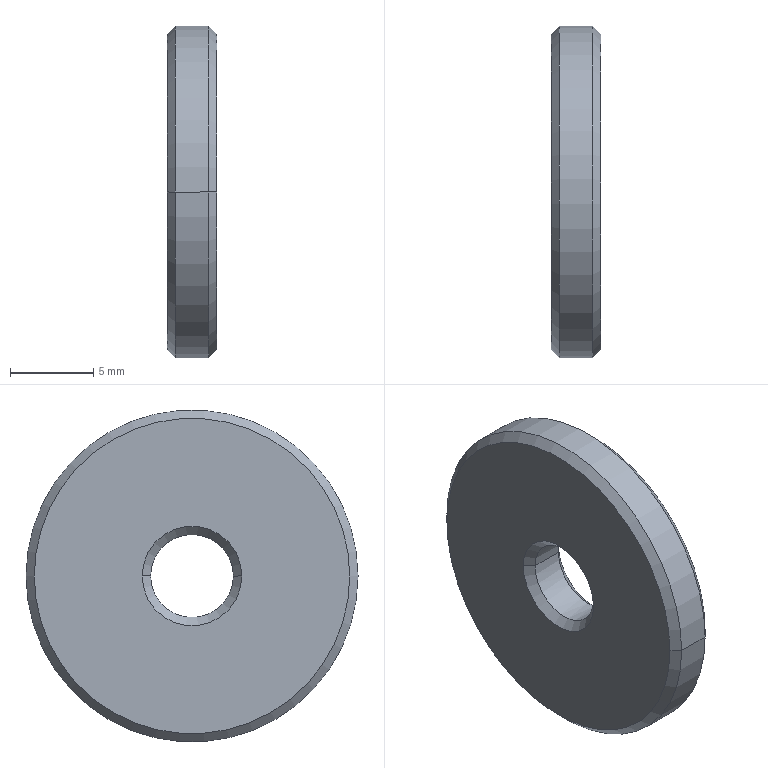Part | STEP file | wssb20_5_3_2_03 | 1 solid | 14 faces | box 3 x 20 x 20 mm | volume 863.938 mm3 | cone 8 | cylinder 4 | plane 2 | commonest cylinder face diameters 5 x2 20 x2
STEP:
#1=CARTESIAN_POINT('',(0.,0.,0.));
#2=DIRECTION('',(0.,0.,1.));
#3=DIRECTION('',(1.,0.,0.));
#4=AXIS2_PLACEMENT_3D('',#1,#2,#3);
#5=CARTESIAN_POINT('',(0.5,-2.5,0.));
#6=VERTEX_POINT('',#5);
#7=CARTESIAN_POINT('',(0.,-3.,0.));
#8=VERTEX_POINT('',#7);
#9=CARTESIAN_POINT('',(0.,-3.,0.));
#10=DIRECTION('',(-0.7071,-0.7071,0.));
#11=VECTOR('',#10,1.);
#12=LINE('',#9,#11);
#13=CARTESIAN_POINT('',(0.,0.,0.));
#14=DIRECTION('',(-1.,0.,0.));
#15=DIRECTION('',(0.,-1.,0.));
#16=AXIS2_PLACEMENT_3D('',#13,#14,#15);
#17=CONICAL_SURFACE('',#16,3.,0.7854);
#18=CARTESIAN_POINT('',(6.283,0.));
#19=DIRECTION('',(0.,1.));
#20=VECTOR('',#19,1.);
#21=LINE('',#18,#20);
#22=(GEOMETRIC_REPRESENTATION_CONTEXT(2)PARAMETRIC_REPRESENTATION_CONTEXT()REPRESENTATION_CONTEXT('',''));
#23=DEFINITIONAL_REPRESENTATION('',(#21),#22);
#24=PCURVE('',#17,#23);
#25=CARTESIAN_POINT('',(0.,0.,0.));
#26=DIRECTION('',(-1.,0.,0.));
#27=DIRECTION('',(0.,-1.,0.));
#28=AXIS2_PLACEMENT_3D('',#25,#26,#27);
#29=CONICAL_SURFACE('',#28,3.,0.7854);
#30=CARTESIAN_POINT('',(0.,0.));
#31=DIRECTION('',(0.,1.));
#32=VECTOR('',#31,1.);
#33=LINE('',#30,#32);
#34=(GEOMETRIC_REPRESENTATION_CONTEXT(2)PARAMETRIC_REPRESENTATION_CONTEXT()REPRESENTATION_CONTEXT('',''));
#35=DEFINITIONAL_REPRESENTATION('',(#33),#34);
#36=PCURVE('',#29,#35);
#37=SURFACE_CURVE('',#12,(#24,#36),.PCURVE_S1.);
#38=EDGE_CURVE('',#6,#8,#37,.T.);
#39=ORIENTED_EDGE('',*,*,#38,.T.);
#40=CARTESIAN_POINT('',(0.,3.,0.));
#41=VERTEX_POINT('',#40);
#42=CARTESIAN_POINT('',(0.,0.,0.));
#43=DIRECTION('',(1.,0.,0.));
#44=DIRECTION('',(0.,-1.,0.));
#45=AXIS2_PLACEMENT_3D('',#42,#43,#44);
#46=CIRCLE('',#45,3.);
#47=CARTESIAN_POINT('',(6.283,0.));
#48=DIRECTION('',(-1.,0.));
#49=VECTOR('',#48,1.);
#50=LINE('',#47,#49);
#51=(GEOMETRIC_REPRESENTATION_CONTEXT(2)PARAMETRIC_REPRESENTATION_CONTEXT()REPRESENTATION_CONTEXT('',''));
#52=DEFINITIONAL_REPRESENTATION('',(#50),#51);
#53=PCURVE('',#17,#52);
#54=CARTESIAN_POINT('',(0.,-6.25,0.));
#55=DIRECTION('',(-1.,0.,0.));
#56=DIRECTION('',(0.,-1.,0.));
#57=AXIS2_PLACEMENT_3D('',#54,#55,#56);
#58=PLANE('',#57);
#59=CARTESIAN_POINT('',(-3.25,0.));
#60=CARTESIAN_POINT('',(-3.25,-5.196));
#61=CARTESIAN_POINT('',(-7.75,-2.598));
#62=CARTESIAN_POINT('',(-12.25,0.));
#63=CARTESIAN_POINT('',(-7.75,2.598));
#64=CARTESIAN_POINT('',(-3.25,5.196));
#65=CARTESIAN_POINT('',(-3.25,0.));
#66=(BOUNDED_CURVE()B_SPLINE_CURVE(2,(#59,#60,#61,#62,#63,#64,#65),.UNSPECIFIED.,.T.,.F.)B_SPLINE_CURVE_WITH_KNOTS((1,2,2,2,2,1),(-2.094,0.,2.094,4.189,6.283,8.378),.UNSPECIFIED.)CURVE()GEOMETRIC_REPRESENTATION_ITEM()RATIONAL_B_SPLINE_CURVE((1.,0.5,1.,0.5,1.,0.5,1.))REPRESENTATION_ITEM(''));
#67=(GEOMETRIC_REPRESENTATION_CONTEXT(2)PARAMETRIC_REPRESENTATION_CONTEXT()REPRESENTATION_CONTEXT('',''));
#68=DEFINITIONAL_REPRESENTATION('',(#66),#67);
#69=PCURVE('',#58,#68);
#70=SURFACE_CURVE('',#46,(#53,#69),.PCURVE_S1.);
#71=EDGE_CURVE('',#8,#41,#70,.T.);
#72=ORIENTED_EDGE('',*,*,#71,.T.);
#73=CARTESIAN_POINT('',(0.5,2.5,0.));
#74=VERTEX_POINT('',#73);
#75=CARTESIAN_POINT('',(0.,3.,0.));
#76=DIRECTION('',(-0.7071,0.7071,0.));
#77=VECTOR('',#76,1.);
#78=LINE('',#75,#77);
#79=CARTESIAN_POINT('',(3.142,0.));
#80=DIRECTION('',(0.,1.));
#81=VECTOR('',#80,1.);
#82=LINE('',#79,#81);
#83=(GEOMETRIC_REPRESENTATION_CONTEXT(2)PARAMETRIC_REPRESENTATION_CONTEXT()REPRESENTATION_CONTEXT('',''));
#84=DEFINITIONAL_REPRESENTATION('',(#82),#83);
#85=PCURVE('',#17,#84);
#86=CARTESIAN_POINT('',(3.142,0.));
#87=DIRECTION('',(0.,1.));
#88=VECTOR('',#87,1.);
#89=LINE('',#86,#88);
#90=(GEOMETRIC_REPRESENTATION_CONTEXT(2)PARAMETRIC_REPRESENTATION_CONTEXT()REPRESENTATION_CONTEXT('',''));
#91=DEFINITIONAL_REPRESENTATION('',(#89),#90);
#92=PCURVE('',#29,#91);
#93=SURFACE_CURVE('',#78,(#85,#92),.PCURVE_S1.);
#94=EDGE_CURVE('',#74,#41,#93,.T.);
#95=ORIENTED_EDGE('',*,*,#94,.F.);
#96=CARTESIAN_POINT('',(0.5,0.,0.));
#97=DIRECTION('',(-1.,0.,0.));
#98=DIRECTION('',(0.,-1.,0.));
#99=AXIS2_PLACEMENT_3D('',#96,#97,#98);
#100=CIRCLE('',#99,2.5);
#101=CARTESIAN_POINT('',(0.,-0.5));
#102=DIRECTION('',(1.,0.));
#103=VECTOR('',#102,1.);
#104=LINE('',#101,#103);
#105=(GEOMETRIC_REPRESENTATION_CONTEXT(2)PARAMETRIC_REPRESENTATION_CONTEXT()REPRESENTATION_CONTEXT('',''));
#106=DEFINITIONAL_REPRESENTATION('',(#104),#105);
#107=PCURVE('',#17,#106);
#108=CARTESIAN_POINT('',(1.5,0.,0.));
#109=DIRECTION('',(-1.,0.,0.));
#110=DIRECTION('',(0.,-1.,0.));
#111=AXIS2_PLACEMENT_3D('',#108,#109,#110);
#112=CYLINDRICAL_SURFACE('',#111,2.5);
#113=CARTESIAN_POINT('',(0.,1.));
#114=DIRECTION('',(1.,0.));
#115=VECTOR('',#114,1.);
#116=LINE('',#113,#115);
#117=(GEOMETRIC_REPRESENTATION_CONTEXT(2)PARAMETRIC_REPRESENTATION_CONTEXT()REPRESENTATION_CONTEXT('',''));
#118=DEFINITIONAL_REPRESENTATION('',(#116),#117);
#119=PCURVE('',#112,#118);
#120=SURFACE_CURVE('',#100,(#107,#119),.PCURVE_S1.);
#121=EDGE_CURVE('',#74,#6,#120,.T.);
#122=ORIENTED_EDGE('',*,*,#121,.T.);
#123=EDGE_LOOP('',(#39,#72,#95,#122));
#124=FACE_BOUND('',#123,.F.);
#125=ADVANCED_FACE('',(#124),#17,.F.);
#126=CARTESIAN_POINT('',(0.,-9.5,0.));
#127=VERTEX_POINT('',#126);
#128=CARTESIAN_POINT('',(0.,9.5,0.));
#129=VERTEX_POINT('',#128);
#130=CARTESIAN_POINT('',(0.,0.,0.));
#131=DIRECTION('',(-1.,0.,0.));
#132=DIRECTION('',(0.,1.,0.));
#133=AXIS2_PLACEMENT_3D('',#130,#131,#132);
#134=CIRCLE('',#133,9.5);
#135=CARTESIAN_POINT('',(0.5,0.,0.));
#136=DIRECTION('',(1.,0.,0.));
#137=DIRECTION('',(0.,1.,0.));
#138=AXIS2_PLACEMENT_3D('',#135,#136,#137);
#139=CONICAL_SURFACE('',#138,10.,0.7854);
#140=CARTESIAN_POINT('',(6.283,-0.5));
#141=DIRECTION('',(-1.,0.));
#142=VECTOR('',#141,1.);
#143=LINE('',#140,#142);
#144=(GEOMETRIC_REPRESENTATION_CONTEXT(2)PARAMETRIC_REPRESENTATION_CONTEXT()REPRESENTATION_CONTEXT('',''));
#145=DEFINITIONAL_REPRESENTATION('',(#143),#144);
#146=PCURVE('',#139,#145);
#147=CARTESIAN_POINT('',(-6.25,0.));
#148=DIRECTION('',(-1.,0.));
#149=AXIS2_PLACEMENT_2D('',#147,#148);
#150=CIRCLE('',#149,9.5);
#151=(GEOMETRIC_REPRESENTATION_CONTEXT(2)PARAMETRIC_REPRESENTATION_CONTEXT()REPRESENTATION_CONTEXT('',''));
#152=DEFINITIONAL_REPRESENTATION('',(#150),#151);
#153=PCURVE('',#58,#152);
#154=SURFACE_CURVE('',#134,(#146,#153),.PCURVE_S1.);
#155=EDGE_CURVE('',#127,#129,#154,.T.);
#156=ORIENTED_EDGE('',*,*,#155,.F.);
#157=CARTESIAN_POINT('',(0.5,-10.,0.));
#158=VERTEX_POINT('',#157);
#159=CARTESIAN_POINT('',(0.5,-10.,0.));
#160=DIRECTION('',(0.7071,-0.7071,0.));
#161=VECTOR('',#160,1.);
#162=LINE('',#159,#161);
#163=CARTESIAN_POINT('',(3.142,0.));
#164=DIRECTION('',(0.,1.));
#165=VECTOR('',#164,1.);
#166=LINE('',#163,#165);
#167=(GEOMETRIC_REPRESENTATION_CONTEXT(2)PARAMETRIC_REPRESENTATION_CONTEXT()REPRESENTATION_CONTEXT('',''));
#168=DEFINITIONAL_REPRESENTATION('',(#166),#167);
#169=PCURVE('',#139,#168);
#170=CARTESIAN_POINT('',(0.5,0.,0.));
#171=DIRECTION('',(1.,0.,0.));
#172=DIRECTION('',(0.,1.,0.));
#173=AXIS2_PLACEMENT_3D('',#170,#171,#172);
#174=CONICAL_SURFACE('',#173,10.,0.7854);
#175=CARTESIAN_POINT('',(3.142,0.));
#176=DIRECTION('',(0.,1.));
#177=VECTOR('',#176,1.);
#178=LINE('',#175,#177);
#179=(GEOMETRIC_REPRESENTATION_CONTEXT(2)PARAMETRIC_REPRESENTATION_CONTEXT()REPRESENTATION_CONTEXT('',''));
#180=DEFINITIONAL_REPRESENTATION('',(#178),#179);
#181=PCURVE('',#174,#180);
#182=SURFACE_CURVE('',#162,(#169,#181),.PCURVE_S1.);
#183=EDGE_CURVE('',#127,#158,#182,.T.);
#184=ORIENTED_EDGE('',*,*,#183,.T.);
#185=CARTESIAN_POINT('',(0.5,10.,0.));
#186=VERTEX_POINT('',#185);
#187=CARTESIAN_POINT('',(0.5,0.,0.));
#188=DIRECTION('',(-1.,0.,0.));
#189=DIRECTION('',(0.,-1.,0.));
#190=AXIS2_PLACEMENT_3D('',#187,#188,#189);
#191=CIRCLE('',#190,10.);
#192=CARTESIAN_POINT('',(3.142,0.));
#193=DIRECTION('',(-1.,0.));
#194=VECTOR('',#193,1.);
#195=LINE('',#192,#194);
#196=(GEOMETRIC_REPRESENTATION_CONTEXT(2)PARAMETRIC_REPRESENTATION_CONTEXT()REPRESENTATION_CONTEXT('',''));
#197=DEFINITIONAL_REPRESENTATION('',(#195),#196);
#198=PCURVE('',#139,#197);
#199=CARTESIAN_POINT('',(1.5,0.,0.));
#200=DIRECTION('',(-1.,0.,0.));
#201=DIRECTION('',(0.,-1.,0.));
#202=AXIS2_PLACEMENT_3D('',#199,#200,#201);
#203=CYLINDRICAL_SURFACE('',#202,10.);
#204=CARTESIAN_POINT('',(0.,1.));
#205=DIRECTION('',(1.,0.));
#206=VECTOR('',#205,1.);
#207=LINE('',#204,#206);
#208=(GEOMETRIC_REPRESENTATION_CONTEXT(2)PARAMETRIC_REPRESENTATION_CONTEXT()REPRESENTATION_CONTEXT('',''));
#209=DEFINITIONAL_REPRESENTATION('',(#207),#208);
#210=PCURVE('',#203,#209);
#211=SURFACE_CURVE('',#191,(#198,#210),.PCURVE_S1.);
#212=EDGE_CURVE('',#158,#186,#211,.T.);
#213=ORIENTED_EDGE('',*,*,#212,.T.);
#214=CARTESIAN_POINT('',(0.5,10.,0.));
#215=DIRECTION('',(0.7071,0.7071,0.));
#216=VECTOR('',#215,1.);
#217=LINE('',#214,#216);
#218=CARTESIAN_POINT('',(0.,0.));
#219=DIRECTION('',(0.,1.));
#220=VECTOR('',#219,1.);
#221=LINE('',#218,#220);
#222=(GEOMETRIC_REPRESENTATION_CONTEXT(2)PARAMETRIC_REPRESENTATION_CONTEXT()REPRESENTATION_CONTEXT('',''));
#223=DEFINITIONAL_REPRESENTATION('',(#221),#222);
#224=PCURVE('',#139,#223);
#225=CARTESIAN_POINT('',(6.283,0.));
#226=DIRECTION('',(0.,1.));
#227=VECTOR('',#226,1.);
#228=LINE('',#225,#227);
#229=(GEOMETRIC_REPRESENTATION_CONTEXT(2)PARAMETRIC_REPRESENTATION_CONTEXT()REPRESENTATION_CONTEXT('',''));
#230=DEFINITIONAL_REPRESENTATION('',(#228),#229);
#231=PCURVE('',#174,#230);
#232=SURFACE_CURVE('',#217,(#224,#231),.PCURVE_S1.);
#233=EDGE_CURVE('',#129,#186,#232,.T.);
#234=ORIENTED_EDGE('',*,*,#233,.F.);
#235=EDGE_LOOP('',(#156,#184,#213,#234));
#236=FACE_BOUND('',#235,.T.);
#237=ADVANCED_FACE('',(#236),#139,.T.);
#238=CARTESIAN_POINT('',(2.5,0.,-2.5));
#239=VERTEX_POINT('',#238);
#240=CARTESIAN_POINT('',(2.5,-2.5,0.));
#241=VERTEX_POINT('',#240);
#242=CARTESIAN_POINT('',(2.5,0.,0.));
#243=DIRECTION('',(-1.,0.,0.));
#244=DIRECTION('',(0.,-1.,0.));
#245=AXIS2_PLACEMENT_3D('',#242,#243,#244);
#246=CIRCLE('',#245,2.5);
#247=CARTESIAN_POINT('',(0.,-1.));
#248=DIRECTION('',(1.,0.));
#249=VECTOR('',#248,1.);
#250=LINE('',#247,#249);
#251=(GEOMETRIC_REPRESENTATION_CONTEXT(2)PARAMETRIC_REPRESENTATION_CONTEXT()REPRESENTATION_CONTEXT('',''));
#252=DEFINITIONAL_REPRESENTATION('',(#250),#251);
#253=PCURVE('',#112,#252);
#254=CARTESIAN_POINT('',(3.,0.,0.));
#255=DIRECTION('',(1.,0.,0.));
#256=DIRECTION('',(0.,0.,-1.));
#257=AXIS2_PLACEMENT_3D('',#254,#255,#256);
#258=CONICAL_SURFACE('',#257,3.,0.7854);
#259=CARTESIAN_POINT('',(10.996,-0.5));
#260=DIRECTION('',(-1.,0.));
#261=VECTOR('',#260,1.);
#262=LINE('',#259,#261);
#263=(GEOMETRIC_REPRESENTATION_CONTEXT(2)PARAMETRIC_REPRESENTATION_CONTEXT()REPRESENTATION_CONTEXT('',''));
#264=DEFINITIONAL_REPRESENTATION('',(#262),#263);
#265=PCURVE('',#258,#264);
#266=SURFACE_CURVE('',#246,(#253,#265),.PCURVE_S1.);
#267=EDGE_CURVE('',#239,#241,#266,.T.);
#268=ORIENTED_EDGE('',*,*,#267,.T.);
#269=CARTESIAN_POINT('',(1.5,-2.5,0.));
#270=DIRECTION('',(-1.,0.,0.));
#271=VECTOR('',#270,1.);
#272=LINE('',#269,#271);
#273=CARTESIAN_POINT('',(6.283,0.));
#274=DIRECTION('',(0.,1.));
#275=VECTOR('',#274,1.);
#276=LINE('',#273,#275);
#277=(GEOMETRIC_REPRESENTATION_CONTEXT(2)PARAMETRIC_REPRESENTATION_CONTEXT()REPRESENTATION_CONTEXT('',''));
#278=DEFINITIONAL_REPRESENTATION('',(#276),#277);
#279=PCURVE('',#112,#278);
#280=CARTESIAN_POINT('',(1.5,0.,0.));
#281=DIRECTION('',(-1.,0.,0.));
#282=DIRECTION('',(0.,-1.,0.));
#283=AXIS2_PLACEMENT_3D('',#280,#281,#282);
#284=CYLINDRICAL_SURFACE('',#283,2.5);
#285=CARTESIAN_POINT('',(0.,0.));
#286=DIRECTION('',(0.,1.));
#287=VECTOR('',#286,1.);
#288=LINE('',#285,#287);
#289=(GEOMETRIC_REPRESENTATION_CONTEXT(2)PARAMETRIC_REPRESENTATION_CONTEXT()REPRESENTATION_CONTEXT('',''));
#290=DEFINITIONAL_REPRESENTATION('',(#288),#289);
#291=PCURVE('',#284,#290);
#292=SURFACE_CURVE('',#272,(#279,#291),.PCURVE_S1.);
#293=EDGE_CURVE('',#241,#6,#292,.T.);
#294=ORIENTED_EDGE('',*,*,#293,.T.);
#295=ORIENTED_EDGE('',*,*,#121,.F.);
#296=CARTESIAN_POINT('',(2.5,2.5,0.));
#297=VERTEX_POINT('',#296);
#298=CARTESIAN_POINT('',(1.5,2.5,0.));
#299=DIRECTION('',(-1.,0.,0.));
#300=VECTOR('',#299,1.);
#301=LINE('',#298,#300);
#302=CARTESIAN_POINT('',(3.142,0.));
#303=DIRECTION('',(0.,1.));
#304=VECTOR('',#303,1.);
#305=LINE('',#302,#304);
#306=(GEOMETRIC_REPRESENTATION_CONTEXT(2)PARAMETRIC_REPRESENTATION_CONTEXT()REPRESENTATION_CONTEXT('',''));
#307=DEFINITIONAL_REPRESENTATION('',(#305),#306);
#308=PCURVE('',#112,#307);
#309=CARTESIAN_POINT('',(3.142,0.));
#310=DIRECTION('',(0.,1.));
#311=VECTOR('',#310,1.);
#312=LINE('',#309,#311);
#313=(GEOMETRIC_REPRESENTATION_CONTEXT(2)PARAMETRIC_REPRESENTATION_CONTEXT()REPRESENTATION_CONTEXT('',''));
#314=DEFINITIONAL_REPRESENTATION('',(#312),#313);
#315=PCURVE('',#284,#314);
#316=SURFACE_CURVE('',#301,(#308,#315),.PCURVE_S1.);
#317=EDGE_CURVE('',#297,#74,#316,.T.);
#318=ORIENTED_EDGE('',*,*,#317,.F.);
#319=CARTESIAN_POINT('',(2.5,0.,0.));
#320=DIRECTION('',(-1.,0.,0.));
#321=DIRECTION('',(0.,-1.,0.));
#322=AXIS2_PLACEMENT_3D('',#319,#320,#321);
#323=CIRCLE('',#322,2.5);
#324=CARTESIAN_POINT('',(0.,-1.));
#325=DIRECTION('',(1.,0.));
#326=VECTOR('',#325,1.);
#327=LINE('',#324,#326);
#328=(GEOMETRIC_REPRESENTATION_CONTEXT(2)PARAMETRIC_REPRESENTATION_CONTEXT()REPRESENTATION_CONTEXT('',''));
#329=DEFINITIONAL_REPRESENTATION('',(#327),#328);
#330=PCURVE('',#112,#329);
#331=CARTESIAN_POINT('',(3.,0.,0.));
#332=DIRECTION('',(1.,0.,0.));
#333=DIRECTION('',(0.,0.,-1.));
#334=AXIS2_PLACEMENT_3D('',#331,#332,#333);
#335=CONICAL_SURFACE('',#334,3.,0.7854);
#336=CARTESIAN_POINT('',(4.712,-0.5));
#337=DIRECTION('',(-1.,0.));
#338=VECTOR('',#337,1.);
#339=LINE('',#336,#338);
#340=(GEOMETRIC_REPRESENTATION_CONTEXT(2)PARAMETRIC_REPRESENTATION_CONTEXT()REPRESENTATION_CONTEXT('',''));
#341=DEFINITIONAL_REPRESENTATION('',(#339),#340);
#342=PCURVE('',#335,#341);
#343=SURFACE_CURVE('',#323,(#330,#342),.PCURVE_S1.);
#344=EDGE_CURVE('',#297,#239,#343,.T.);
#345=ORIENTED_EDGE('',*,*,#344,.T.);
#346=EDGE_LOOP('',(#268,#294,#295,#318,#345));
#347=FACE_BOUND('',#346,.F.);
#348=ADVANCED_FACE('',(#347),#112,.F.);
#349=CARTESIAN_POINT('',(2.5,-10.,0.));
#350=VERTEX_POINT('',#349);
#351=CARTESIAN_POINT('',(2.5,10.,0.));
#352=VERTEX_POINT('',#351);
#353=CARTESIAN_POINT('',(2.5,0.,0.));
#354=DIRECTION('',(-1.,0.,0.));
#355=DIRECTION('',(0.,-1.,0.));
#356=AXIS2_PLACEMENT_3D('',#353,#354,#355);
#357=CIRCLE('',#356,10.);
#358=CARTESIAN_POINT('',(0.,-1.));
#359=DIRECTION('',(1.,0.));
#360=VECTOR('',#359,1.);
#361=LINE('',#358,#360);
#362=(GEOMETRIC_REPRESENTATION_CONTEXT(2)PARAMETRIC_REPRESENTATION_CONTEXT()REPRESENTATION_CONTEXT('',''));
#363=DEFINITIONAL_REPRESENTATION('',(#361),#362);
#364=PCURVE('',#203,#363);
#365=CARTESIAN_POINT('',(2.5,0.,0.));
#366=DIRECTION('',(-1.,0.,0.));
#367=DIRECTION('',(0.,-1.,0.));
#368=AXIS2_PLACEMENT_3D('',#365,#366,#367);
#369=CONICAL_SURFACE('',#368,10.,0.7854);
#370=CARTESIAN_POINT('',(0.,0.));
#371=DIRECTION('',(1.,0.));
#372=VECTOR('',#371,1.);
#373=LINE('',#370,#372);
#374=(GEOMETRIC_REPRESENTATION_CONTEXT(2)PARAMETRIC_REPRESENTATION_CONTEXT()REPRESENTATION_CONTEXT('',''));
#375=DEFINITIONAL_REPRESENTATION('',(#373),#374);
#376=PCURVE('',#369,#375);
#377=SURFACE_CURVE('',#357,(#364,#376),.PCURVE_S1.);
#378=EDGE_CURVE('',#350,#352,#377,.T.);
#379=ORIENTED_EDGE('',*,*,#378,.T.);
#380=CARTESIAN_POINT('',(1.5,10.,0.));
#381=DIRECTION('',(-1.,0.,0.));
#382=VECTOR('',#381,1.);
#383=LINE('',#380,#382);
#384=CARTESIAN_POINT('',(3.142,0.));
#385=DIRECTION('',(0.,1.));
#386=VECTOR('',#385,1.);
#387=LINE('',#384,#386);
#388=(GEOMETRIC_REPRESENTATION_CONTEXT(2)PARAMETRIC_REPRESENTATION_CONTEXT()REPRESENTATION_CONTEXT('',''));
#389=DEFINITIONAL_REPRESENTATION('',(#387),#388);
#390=PCURVE('',#203,#389);
#391=CARTESIAN_POINT('',(1.5,0.,0.));
#392=DIRECTION('',(-1.,0.,0.));
#393=DIRECTION('',(0.,-1.,0.));
#394=AXIS2_PLACEMENT_3D('',#391,#392,#393);
#395=CYLINDRICAL_SURFACE('',#394,10.);
#396=CARTESIAN_POINT('',(3.142,0.));
#397=DIRECTION('',(0.,1.));
#398=VECTOR('',#397,1.);
#399=LINE('',#396,#398);
#400=(GEOMETRIC_REPRESENTATION_CONTEXT(2)PARAMETRIC_REPRESENTATION_CONTEXT()REPRESENTATION_CONTEXT('',''));
#401=DEFINITIONAL_REPRESENTATION('',(#399),#400);
#402=PCURVE('',#395,#401);
#403=SURFACE_CURVE('',#383,(#390,#402),.PCURVE_S1.);
#404=EDGE_CURVE('',#352,#186,#403,.T.);
#405=ORIENTED_EDGE('',*,*,#404,.T.);
#406=ORIENTED_EDGE('',*,*,#212,.F.);
#407=CARTESIAN_POINT('',(1.5,-10.,0.));
#408=DIRECTION('',(-1.,0.,0.));
#409=VECTOR('',#408,1.);
#410=LINE('',#407,#409);
#411=CARTESIAN_POINT('',(0.,0.));
#412=DIRECTION('',(0.,1.));
#413=VECTOR('',#412,1.);
#414=LINE('',#411,#413);
#415=(GEOMETRIC_REPRESENTATION_CONTEXT(2)PARAMETRIC_REPRESENTATION_CONTEXT()REPRESENTATION_CONTEXT('',''));
#416=DEFINITIONAL_REPRESENTATION('',(#414),#415);
#417=PCURVE('',#203,#416);
#418=CARTESIAN_POINT('',(6.283,0.));
#419=DIRECTION('',(0.,1.));
#420=VECTOR('',#419,1.);
#421=LINE('',#418,#420);
#422=(GEOMETRIC_REPRESENTATION_CONTEXT(2)PARAMETRIC_REPRESENTATION_CONTEXT()REPRESENTATION_CONTEXT('',''));
#423=DEFINITIONAL_REPRESENTATION('',(#421),#422);
#424=PCURVE('',#395,#423);
#425=SURFACE_CURVE('',#410,(#417,#424),.PCURVE_S1.);
#426=EDGE_CURVE('',#350,#158,#425,.T.);
#427=ORIENTED_EDGE('',*,*,#426,.F.);
#428=EDGE_LOOP('',(#379,#405,#406,#427));
#429=FACE_BOUND('',#428,.T.);
#430=ADVANCED_FACE('',(#429),#203,.T.);
#431=CARTESIAN_POINT('',(3.,0.,-3.));
#432=VERTEX_POINT('',#431);
#433=CARTESIAN_POINT('',(3.,0.,-3.));
#434=DIRECTION('',(0.7071,0.,-0.7071));
#435=VECTOR('',#434,1.);
#436=LINE('',#433,#435);
#437=CARTESIAN_POINT('',(6.283,0.));
#438=DIRECTION('',(0.,1.));
#439=VECTOR('',#438,1.);
#440=LINE('',#437,#439);
#441=(GEOMETRIC_REPRESENTATION_CONTEXT(2)PARAMETRIC_REPRESENTATION_CONTEXT()REPRESENTATION_CONTEXT('',''));
#442=DEFINITIONAL_REPRESENTATION('',(#440),#441);
#443=PCURVE('',#258,#442);
#444=CARTESIAN_POINT('',(0.,0.));
#445=DIRECTION('',(0.,1.));
#446=VECTOR('',#445,1.);
#447=LINE('',#444,#446);
#448=(GEOMETRIC_REPRESENTATION_CONTEXT(2)PARAMETRIC_REPRESENTATION_CONTEXT()REPRESENTATION_CONTEXT('',''));
#449=DEFINITIONAL_REPRESENTATION('',(#447),#448);
#450=PCURVE('',#335,#449);
#451=SURFACE_CURVE('',#436,(#443,#450),.PCURVE_S1.);
#452=EDGE_CURVE('',#239,#432,#451,.T.);
#453=ORIENTED_EDGE('',*,*,#452,.T.);
#454=CARTESIAN_POINT('',(3.,0.,3.));
#455=VERTEX_POINT('',#454);
#456=CARTESIAN_POINT('',(3.,0.,0.));
#457=DIRECTION('',(-1.,0.,0.));
#458=DIRECTION('',(0.,0.,-1.));
#459=AXIS2_PLACEMENT_3D('',#456,#457,#458);
#460=CIRCLE('',#459,3.);
#461=CARTESIAN_POINT('',(6.283,0.));
#462=DIRECTION('',(-1.,0.));
#463=VECTOR('',#462,1.);
#464=LINE('',#461,#463);
#465=(GEOMETRIC_REPRESENTATION_CONTEXT(2)PARAMETRIC_REPRESENTATION_CONTEXT()REPRESENTATION_CONTEXT('',''));
#466=DEFINITIONAL_REPRESENTATION('',(#464),#465);
#467=PCURVE('',#258,#466);
#468=CARTESIAN_POINT('',(3.,-6.25,0.));
#469=DIRECTION('',(1.,0.,0.));
#470=DIRECTION('',(0.,1.,0.));
#471=AXIS2_PLACEMENT_3D('',#468,#469,#470);
#472=PLANE('',#471);
#473=CARTESIAN_POINT('',(6.25,-3.));
#474=CARTESIAN_POINT('',(1.054,-3.));
#475=CARTESIAN_POINT('',(3.652,1.5));
#476=CARTESIAN_POINT('',(6.25,6.));
#477=CARTESIAN_POINT('',(8.848,1.5));
#478=CARTESIAN_POINT('',(11.446,-3.));
#479=CARTESIAN_POINT('',(6.25,-3.));
#480=(BOUNDED_CURVE()B_SPLINE_CURVE(2,(#473,#474,#475,#476,#477,#478,#479),.UNSPECIFIED.,.T.,.F.)B_SPLINE_CURVE_WITH_KNOTS((1,2,2,2,2,1),(-2.094,0.,2.094,4.189,6.283,8.378),.UNSPECIFIED.)CURVE()GEOMETRIC_REPRESENTATION_ITEM()RATIONAL_B_SPLINE_CURVE((1.,0.5,1.,0.5,1.,0.5,1.))REPRESENTATION_ITEM(''));
#481=(GEOMETRIC_REPRESENTATION_CONTEXT(2)PARAMETRIC_REPRESENTATION_CONTEXT()REPRESENTATION_CONTEXT('',''));
#482=DEFINITIONAL_REPRESENTATION('',(#480),#481);
#483=PCURVE('',#472,#482);
#484=SURFACE_CURVE('',#460,(#467,#483),.PCURVE_S1.);
#485=EDGE_CURVE('',#432,#455,#484,.T.);
#486=ORIENTED_EDGE('',*,*,#485,.T.);
#487=CARTESIAN_POINT('',(2.5,0.,2.5));
#488=VERTEX_POINT('',#487);
#489=CARTESIAN_POINT('',(3.,0.,3.));
#490=DIRECTION('',(0.7071,0.,0.7071));
#491=VECTOR('',#490,1.);
#492=LINE('',#489,#491);
#493=CARTESIAN_POINT('',(3.142,0.));
#494=DIRECTION('',(0.,1.));
#495=VECTOR('',#494,1.);
#496=LINE('',#493,#495);
#497=(GEOMETRIC_REPRESENTATION_CONTEXT(2)PARAMETRIC_REPRESENTATION_CONTEXT()REPRESENTATION_CONTEXT('',''));
#498=DEFINITIONAL_REPRESENTATION('',(#496),#497);
#499=PCURVE('',#258,#498);
#500=CARTESIAN_POINT('',(3.142,0.));
#501=DIRECTION('',(0.,1.));
#502=VECTOR('',#501,1.);
#503=LINE('',#500,#502);
#504=(GEOMETRIC_REPRESENTATION_CONTEXT(2)PARAMETRIC_REPRESENTATION_CONTEXT()REPRESENTATION_CONTEXT('',''));
#505=DEFINITIONAL_REPRESENTATION('',(#503),#504);
#506=PCURVE('',#335,#505);
#507=SURFACE_CURVE('',#492,(#499,#506),.PCURVE_S1.);
#508=EDGE_CURVE('',#488,#455,#507,.T.);
#509=ORIENTED_EDGE('',*,*,#508,.F.);
#510=CARTESIAN_POINT('',(2.5,0.,0.));
#511=DIRECTION('',(-1.,0.,0.));
#512=DIRECTION('',(0.,-1.,0.));
#513=AXIS2_PLACEMENT_3D('',#510,#511,#512);
#514=CIRCLE('',#513,2.5);
#515=CARTESIAN_POINT('',(4.712,-0.5));
#516=DIRECTION('',(-1.,0.));
#517=VECTOR('',#516,1.);
#518=LINE('',#515,#517);
#519=(GEOMETRIC_REPRESENTATION_CONTEXT(2)PARAMETRIC_REPRESENTATION_CONTEXT()REPRESENTATION_CONTEXT('',''));
#520=DEFINITIONAL_REPRESENTATION('',(#518),#519);
#521=PCURVE('',#258,#520);
#522=CARTESIAN_POINT('',(0.,-1.));
#523=DIRECTION('',(1.,0.));
#524=VECTOR('',#523,1.);
#525=LINE('',#522,#524);
#526=(GEOMETRIC_REPRESENTATION_CONTEXT(2)PARAMETRIC_REPRESENTATION_CONTEXT()REPRESENTATION_CONTEXT('',''));
#527=DEFINITIONAL_REPRESENTATION('',(#525),#526);
#528=PCURVE('',#284,#527);
#529=SURFACE_CURVE('',#514,(#521,#528),.PCURVE_S1.);
#530=EDGE_CURVE('',#241,#488,#529,.T.);
#531=ORIENTED_EDGE('',*,*,#530,.F.);
#532=ORIENTED_EDGE('',*,*,#267,.F.);
#533=EDGE_LOOP('',(#453,#486,#509,#531,#532));
#534=FACE_BOUND('',#533,.F.);
#535=ADVANCED_FACE('',(#534),#258,.F.);
#536=CARTESIAN_POINT('',(3.,-9.5,0.));
#537=VERTEX_POINT('',#536);
#538=CARTESIAN_POINT('',(3.,9.5,0.));
#539=VERTEX_POINT('',#538);
#540=CARTESIAN_POINT('',(3.,0.,0.));
#541=DIRECTION('',(-1.,0.,0.));
#542=DIRECTION('',(0.,-1.,0.));
#543=AXIS2_PLACEMENT_3D('',#540,#541,#542);
#544=CIRCLE('',#543,9.5);
#545=CARTESIAN_POINT('',(0.,-0.5));
#546=DIRECTION('',(1.,0.));
#547=VECTOR('',#546,1.);
#548=LINE('',#545,#547);
#549=(GEOMETRIC_REPRESENTATION_CONTEXT(2)PARAMETRIC_REPRESENTATION_CONTEXT()REPRESENTATION_CONTEXT('',''));
#550=DEFINITIONAL_REPRESENTATION('',(#548),#549);
#551=PCURVE('',#369,#550);
#552=CARTESIAN_POINT('',(-3.25,0.));
#553=CARTESIAN_POINT('',(-3.25,16.454));
#554=CARTESIAN_POINT('',(11.,8.227));
#555=CARTESIAN_POINT('',(25.25,0.));
#556=CARTESIAN_POINT('',(11.,-8.227));
#557=CARTESIAN_POINT('',(-3.25,-16.454));
#558=CARTESIAN_POINT('',(-3.25,0.));
#559=(BOUNDED_CURVE()B_SPLINE_CURVE(2,(#552,#553,#554,#555,#556,#557,#558),.UNSPECIFIED.,.T.,.F.)B_SPLINE_CURVE_WITH_KNOTS((1,2,2,2,2,1),(-2.094,0.,2.094,4.189,6.283,8.378),.UNSPECIFIED.)CURVE()GEOMETRIC_REPRESENTATION_ITEM()RATIONAL_B_SPLINE_CURVE((1.,0.5,1.,0.5,1.,0.5,1.))REPRESENTATION_ITEM(''));
#560=(GEOMETRIC_REPRESENTATION_CONTEXT(2)PARAMETRIC_REPRESENTATION_CONTEXT()REPRESENTATION_CONTEXT('',''));
#561=DEFINITIONAL_REPRESENTATION('',(#559),#560);
#562=PCURVE('',#472,#561);
#563=SURFACE_CURVE('',#544,(#551,#562),.PCURVE_S1.);
#564=EDGE_CURVE('',#537,#539,#563,.T.);
#565=ORIENTED_EDGE('',*,*,#564,.T.);
#566=CARTESIAN_POINT('',(2.5,10.,0.));
#567=DIRECTION('',(-0.7071,0.7071,0.));
#568=VECTOR('',#567,1.);
#569=LINE('',#566,#568);
#570=CARTESIAN_POINT('',(3.142,0.));
#571=DIRECTION('',(0.,1.));
#572=VECTOR('',#571,1.);
#573=LINE('',#570,#572);
#574=(GEOMETRIC_REPRESENTATION_CONTEXT(2)PARAMETRIC_REPRESENTATION_CONTEXT()REPRESENTATION_CONTEXT('',''));
#575=DEFINITIONAL_REPRESENTATION('',(#573),#574);
#576=PCURVE('',#369,#575);
#577=CARTESIAN_POINT('',(2.5,0.,0.));
#578=DIRECTION('',(-1.,0.,0.));
#579=DIRECTION('',(0.,-1.,0.));
#580=AXIS2_PLACEMENT_3D('',#577,#578,#579);
#581=CONICAL_SURFACE('',#580,10.,0.7854);
#582=CARTESIAN_POINT('',(3.142,0.));
#583=DIRECTION('',(0.,1.));
#584=VECTOR('',#583,1.);
#585=LINE('',#582,#584);
#586=(GEOMETRIC_REPRESENTATION_CONTEXT(2)PARAMETRIC_REPRESENTATION_CONTEXT()REPRESENTATION_CONTEXT('',''));
#587=DEFINITIONAL_REPRESENTATION('',(#585),#586);
#588=PCURVE('',#581,#587);
#589=SURFACE_CURVE('',#569,(#576,#588),.PCURVE_S1.);
#590=EDGE_CURVE('',#539,#352,#589,.T.);
#591=ORIENTED_EDGE('',*,*,#590,.T.);
#592=ORIENTED_EDGE('',*,*,#378,.F.);
#593=CARTESIAN_POINT('',(2.5,-10.,0.));
#594=DIRECTION('',(-0.7071,-0.7071,0.));
#595=VECTOR('',#594,1.);
#596=LINE('',#593,#595);
#597=CARTESIAN_POINT('',(0.,0.));
#598=DIRECTION('',(0.,1.));
#599=VECTOR('',#598,1.);
#600=LINE('',#597,#599);
#601=(GEOMETRIC_REPRESENTATION_CONTEXT(2)PARAMETRIC_REPRESENTATION_CONTEXT()REPRESENTATION_CONTEXT('',''));
#602=DEFINITIONAL_REPRESENTATION('',(#600),#601);
#603=PCURVE('',#369,#602);
#604=CARTESIAN_POINT('',(6.283,0.));
#605=DIRECTION('',(0.,1.));
#606=VECTOR('',#605,1.);
#607=LINE('',#604,#606);
#608=(GEOMETRIC_REPRESENTATION_CONTEXT(2)PARAMETRIC_REPRESENTATION_CONTEXT()REPRESENTATION_CONTEXT('',''));
#609=DEFINITIONAL_REPRESENTATION('',(#607),#608);
#610=PCURVE('',#581,#609);
#611=SURFACE_CURVE('',#596,(#603,#610),.PCURVE_S1.);
#612=EDGE_CURVE('',#537,#350,#611,.T.);
#613=ORIENTED_EDGE('',*,*,#612,.F.);
#614=EDGE_LOOP('',(#565,#591,#592,#613));
#615=FACE_BOUND('',#614,.T.);
#616=ADVANCED_FACE('',(#615),#369,.T.);
#617=ORIENTED_EDGE('',*,*,#71,.T.);
#618=CARTESIAN_POINT('',(0.,0.,0.));
#619=DIRECTION('',(1.,0.,0.));
#620=DIRECTION('',(0.,-1.,0.));
#621=AXIS2_PLACEMENT_3D('',#618,#619,#620);
#622=CIRCLE('',#621,3.);
#623=CARTESIAN_POINT('',(-3.25,0.));
#624=CARTESIAN_POINT('',(-3.25,-5.196));
#625=CARTESIAN_POINT('',(-7.75,-2.598));
#626=CARTESIAN_POINT('',(-12.25,0.));
#627=CARTESIAN_POINT('',(-7.75,2.598));
#628=CARTESIAN_POINT('',(-3.25,5.196));
#629=CARTESIAN_POINT('',(-3.25,0.));
#630=(BOUNDED_CURVE()B_SPLINE_CURVE(2,(#623,#624,#625,#626,#627,#628,#629),.UNSPECIFIED.,.T.,.F.)B_SPLINE_CURVE_WITH_KNOTS((1,2,2,2,2,1),(-2.094,0.,2.094,4.189,6.283,8.378),.UNSPECIFIED.)CURVE()GEOMETRIC_REPRESENTATION_ITEM()RATIONAL_B_SPLINE_CURVE((1.,0.5,1.,0.5,1.,0.5,1.))REPRESENTATION_ITEM(''));
#631=(GEOMETRIC_REPRESENTATION_CONTEXT(2)PARAMETRIC_REPRESENTATION_CONTEXT()REPRESENTATION_CONTEXT('',''));
#632=DEFINITIONAL_REPRESENTATION('',(#630),#631);
#633=PCURVE('',#58,#632);
#634=CARTESIAN_POINT('',(6.283,0.));
#635=DIRECTION('',(-1.,0.));
#636=VECTOR('',#635,1.);
#637=LINE('',#634,#636);
#638=(GEOMETRIC_REPRESENTATION_CONTEXT(2)PARAMETRIC_REPRESENTATION_CONTEXT()REPRESENTATION_CONTEXT('',''));
#639=DEFINITIONAL_REPRESENTATION('',(#637),#638);
#640=PCURVE('',#29,#639);
#641=SURFACE_CURVE('',#622,(#633,#640),.PCURVE_S1.);
#642=EDGE_CURVE('',#41,#8,#641,.T.);
#643=ORIENTED_EDGE('',*,*,#642,.T.);
#644=EDGE_LOOP('',(#617,#643));
#645=FACE_BOUND('',#644,.T.);
#646=CARTESIAN_POINT('',(0.,0.,0.));
#647=DIRECTION('',(-1.,0.,0.));
#648=DIRECTION('',(0.,1.,0.));
#649=AXIS2_PLACEMENT_3D('',#646,#647,#648);
#650=CIRCLE('',#649,9.5);
#651=CARTESIAN_POINT('',(-6.25,0.));
#652=DIRECTION('',(-1.,0.));
#653=AXIS2_PLACEMENT_2D('',#651,#652);
#654=CIRCLE('',#653,9.5);
#655=(GEOMETRIC_REPRESENTATION_CONTEXT(2)PARAMETRIC_REPRESENTATION_CONTEXT()REPRESENTATION_CONTEXT('',''));
#656=DEFINITIONAL_REPRESENTATION('',(#654),#655);
#657=PCURVE('',#58,#656);
#658=CARTESIAN_POINT('',(6.283,-0.5));
#659=DIRECTION('',(-1.,0.));
#660=VECTOR('',#659,1.);
#661=LINE('',#658,#660);
#662=(GEOMETRIC_REPRESENTATION_CONTEXT(2)PARAMETRIC_REPRESENTATION_CONTEXT()REPRESENTATION_CONTEXT('',''));
#663=DEFINITIONAL_REPRESENTATION('',(#661),#662);
#664=PCURVE('',#174,#663);
#665=SURFACE_CURVE('',#650,(#657,#664),.PCURVE_S1.);
#666=EDGE_CURVE('',#129,#127,#665,.T.);
#667=ORIENTED_EDGE('',*,*,#666,.T.);
#668=ORIENTED_EDGE('',*,*,#155,.T.);
#669=EDGE_LOOP('',(#667,#668));
#670=FACE_BOUND('',#669,.T.);
#671=ADVANCED_FACE('',(#645,#670),#58,.T.);
#672=ORIENTED_EDGE('',*,*,#642,.T.);
#673=ORIENTED_EDGE('',*,*,#38,.F.);
#674=CARTESIAN_POINT('',(0.5,0.,0.));
#675=DIRECTION('',(-1.,0.,0.));
#676=DIRECTION('',(0.,-1.,0.));
#677=AXIS2_PLACEMENT_3D('',#674,#675,#676);
#678=CIRCLE('',#677,2.5);
#679=CARTESIAN_POINT('',(0.,-0.5));
#680=DIRECTION('',(1.,0.));
#681=VECTOR('',#680,1.);
#682=LINE('',#679,#681);
#683=(GEOMETRIC_REPRESENTATION_CONTEXT(2)PARAMETRIC_REPRESENTATION_CONTEXT()REPRESENTATION_CONTEXT('',''));
#684=DEFINITIONAL_REPRESENTATION('',(#682),#683);
#685=PCURVE('',#29,#684);
#686=CARTESIAN_POINT('',(0.,1.));
#687=DIRECTION('',(1.,0.));
#688=VECTOR('',#687,1.);
#689=LINE('',#686,#688);
#690=(GEOMETRIC_REPRESENTATION_CONTEXT(2)PARAMETRIC_REPRESENTATION_CONTEXT()REPRESENTATION_CONTEXT('',''));
#691=DEFINITIONAL_REPRESENTATION('',(#689),#690);
#692=PCURVE('',#284,#691);
#693=SURFACE_CURVE('',#678,(#685,#692),.PCURVE_S1.);
#694=EDGE_CURVE('',#6,#74,#693,.T.);
#695=ORIENTED_EDGE('',*,*,#694,.T.);
#696=ORIENTED_EDGE('',*,*,#94,.T.);
#697=EDGE_LOOP('',(#672,#673,#695,#696));
#698=FACE_BOUND('',#697,.F.);
#699=ADVANCED_FACE('',(#698),#29,.F.);
#700=ORIENTED_EDGE('',*,*,#183,.F.);
#701=ORIENTED_EDGE('',*,*,#666,.F.);
#702=ORIENTED_EDGE('',*,*,#233,.T.);
#703=CARTESIAN_POINT('',(0.5,0.,0.));
#704=DIRECTION('',(-1.,0.,0.));
#705=DIRECTION('',(0.,-1.,0.));
#706=AXIS2_PLACEMENT_3D('',#703,#704,#705);
#707=CIRCLE('',#706,10.);
#708=CARTESIAN_POINT('',(9.425,0.));
#709=DIRECTION('',(-1.,0.));
#710=VECTOR('',#709,1.);
#711=LINE('',#708,#710);
#712=(GEOMETRIC_REPRESENTATION_CONTEXT(2)PARAMETRIC_REPRESENTATION_CONTEXT()REPRESENTATION_CONTEXT('',''));
#713=DEFINITIONAL_REPRESENTATION('',(#711),#712);
#714=PCURVE('',#174,#713);
#715=CARTESIAN_POINT('',(0.,1.));
#716=DIRECTION('',(1.,0.));
#717=VECTOR('',#716,1.);
#718=LINE('',#715,#717);
#719=(GEOMETRIC_REPRESENTATION_CONTEXT(2)PARAMETRIC_REPRESENTATION_CONTEXT()REPRESENTATION_CONTEXT('',''));
#720=DEFINITIONAL_REPRESENTATION('',(#718),#719);
#721=PCURVE('',#395,#720);
#722=SURFACE_CURVE('',#707,(#714,#721),.PCURVE_S1.);
#723=EDGE_CURVE('',#186,#158,#722,.T.);
#724=ORIENTED_EDGE('',*,*,#723,.T.);
#725=EDGE_LOOP('',(#700,#701,#702,#724));
#726=FACE_BOUND('',#725,.T.);
#727=ADVANCED_FACE('',(#726),#174,.T.);
#728=ORIENTED_EDGE('',*,*,#694,.F.);
#729=ORIENTED_EDGE('',*,*,#293,.F.);
#730=ORIENTED_EDGE('',*,*,#530,.T.);
#731=CARTESIAN_POINT('',(2.5,0.,0.));
#732=DIRECTION('',(-1.,0.,0.));
#733=DIRECTION('',(0.,-1.,0.));
#734=AXIS2_PLACEMENT_3D('',#731,#732,#733);
#735=CIRCLE('',#734,2.5);
#736=CARTESIAN_POINT('',(0.,-1.));
#737=DIRECTION('',(1.,0.));
#738=VECTOR('',#737,1.);
#739=LINE('',#736,#738);
#740=(GEOMETRIC_REPRESENTATION_CONTEXT(2)PARAMETRIC_REPRESENTATION_CONTEXT()REPRESENTATION_CONTEXT('',''));
#741=DEFINITIONAL_REPRESENTATION('',(#739),#740);
#742=PCURVE('',#284,#741);
#743=CARTESIAN_POINT('',(4.712,-0.5));
#744=DIRECTION('',(-1.,0.));
#745=VECTOR('',#744,1.);
#746=LINE('',#743,#745);
#747=(GEOMETRIC_REPRESENTATION_CONTEXT(2)PARAMETRIC_REPRESENTATION_CONTEXT()REPRESENTATION_CONTEXT('',''));
#748=DEFINITIONAL_REPRESENTATION('',(#746),#747);
#749=PCURVE('',#335,#748);
#750=SURFACE_CURVE('',#735,(#742,#749),.PCURVE_S1.);
#751=EDGE_CURVE('',#488,#297,#750,.T.);
#752=ORIENTED_EDGE('',*,*,#751,.T.);
#753=ORIENTED_EDGE('',*,*,#317,.T.);
#754=EDGE_LOOP('',(#728,#729,#730,#752,#753));
#755=FACE_BOUND('',#754,.F.);
#756=ADVANCED_FACE('',(#755),#284,.F.);
#757=ORIENTED_EDGE('',*,*,#404,.F.);
#758=CARTESIAN_POINT('',(2.5,0.,0.));
#759=DIRECTION('',(-1.,0.,0.));
#760=DIRECTION('',(0.,-1.,0.));
#761=AXIS2_PLACEMENT_3D('',#758,#759,#760);
#762=CIRCLE('',#761,10.);
#763=CARTESIAN_POINT('',(0.,-1.));
#764=DIRECTION('',(1.,0.));
#765=VECTOR('',#764,1.);
#766=LINE('',#763,#765);
#767=(GEOMETRIC_REPRESENTATION_CONTEXT(2)PARAMETRIC_REPRESENTATION_CONTEXT()REPRESENTATION_CONTEXT('',''));
#768=DEFINITIONAL_REPRESENTATION('',(#766),#767);
#769=PCURVE('',#395,#768);
#770=CARTESIAN_POINT('',(0.,0.));
#771=DIRECTION('',(1.,0.));
#772=VECTOR('',#771,1.);
#773=LINE('',#770,#772);
#774=(GEOMETRIC_REPRESENTATION_CONTEXT(2)PARAMETRIC_REPRESENTATION_CONTEXT()REPRESENTATION_CONTEXT('',''));
#775=DEFINITIONAL_REPRESENTATION('',(#773),#774);
#776=PCURVE('',#581,#775);
#777=SURFACE_CURVE('',#762,(#769,#776),.PCURVE_S1.);
#778=EDGE_CURVE('',#352,#350,#777,.T.);
#779=ORIENTED_EDGE('',*,*,#778,.T.);
#780=ORIENTED_EDGE('',*,*,#426,.T.);
#781=ORIENTED_EDGE('',*,*,#723,.F.);
#782=EDGE_LOOP('',(#757,#779,#780,#781));
#783=FACE_BOUND('',#782,.T.);
#784=ADVANCED_FACE('',(#783),#395,.T.);
#785=CARTESIAN_POINT('',(3.,0.,0.));
#786=DIRECTION('',(-1.,0.,0.));
#787=DIRECTION('',(0.,0.,-1.));
#788=AXIS2_PLACEMENT_3D('',#785,#786,#787);
#789=CIRCLE('',#788,3.);
#790=CARTESIAN_POINT('',(6.283,0.));
#791=DIRECTION('',(-1.,0.));
#792=VECTOR('',#791,1.);
#793=LINE('',#790,#792);
#794=(GEOMETRIC_REPRESENTATION_CONTEXT(2)PARAMETRIC_REPRESENTATION_CONTEXT()REPRESENTATION_CONTEXT('',''));
#795=DEFINITIONAL_REPRESENTATION('',(#793),#794);
#796=PCURVE('',#335,#795);
#797=CARTESIAN_POINT('',(6.25,-3.));
#798=CARTESIAN_POINT('',(1.054,-3.));
#799=CARTESIAN_POINT('',(3.652,1.5));
#800=CARTESIAN_POINT('',(6.25,6.));
#801=CARTESIAN_POINT('',(8.848,1.5));
#802=CARTESIAN_POINT('',(11.446,-3.));
#803=CARTESIAN_POINT('',(6.25,-3.));
#804=(BOUNDED_CURVE()B_SPLINE_CURVE(2,(#797,#798,#799,#800,#801,#802,#803),.UNSPECIFIED.,.T.,.F.)B_SPLINE_CURVE_WITH_KNOTS((1,2,2,2,2,1),(-2.094,0.,2.094,4.189,6.283,8.378),.UNSPECIFIED.)CURVE()GEOMETRIC_REPRESENTATION_ITEM()RATIONAL_B_SPLINE_CURVE((1.,0.5,1.,0.5,1.,0.5,1.))REPRESENTATION_ITEM(''));
#805=(GEOMETRIC_REPRESENTATION_CONTEXT(2)PARAMETRIC_REPRESENTATION_CONTEXT()REPRESENTATION_CONTEXT('',''));
#806=DEFINITIONAL_REPRESENTATION('',(#804),#805);
#807=PCURVE('',#472,#806);
#808=SURFACE_CURVE('',#789,(#796,#807),.PCURVE_S1.);
#809=EDGE_CURVE('',#455,#432,#808,.T.);
#810=ORIENTED_EDGE('',*,*,#809,.T.);
#811=ORIENTED_EDGE('',*,*,#452,.F.);
#812=ORIENTED_EDGE('',*,*,#344,.F.);
#813=ORIENTED_EDGE('',*,*,#751,.F.);
#814=ORIENTED_EDGE('',*,*,#508,.T.);
#815=EDGE_LOOP('',(#810,#811,#812,#813,#814));
#816=FACE_BOUND('',#815,.F.);
#817=ADVANCED_FACE('',(#816),#335,.F.);
#818=ORIENTED_EDGE('',*,*,#590,.F.);
#819=CARTESIAN_POINT('',(3.,0.,0.));
#820=DIRECTION('',(-1.,0.,0.));
#821=DIRECTION('',(0.,-1.,0.));
#822=AXIS2_PLACEMENT_3D('',#819,#820,#821);
#823=CIRCLE('',#822,9.5);
#824=CARTESIAN_POINT('',(0.,-0.5));
#825=DIRECTION('',(1.,0.));
#826=VECTOR('',#825,1.);
#827=LINE('',#824,#826);
#828=(GEOMETRIC_REPRESENTATION_CONTEXT(2)PARAMETRIC_REPRESENTATION_CONTEXT()REPRESENTATION_CONTEXT('',''));
#829=DEFINITIONAL_REPRESENTATION('',(#827),#828);
#830=PCURVE('',#581,#829);
#831=CARTESIAN_POINT('',(-3.25,0.));
#832=CARTESIAN_POINT('',(-3.25,16.454));
#833=CARTESIAN_POINT('',(11.,8.227));
#834=CARTESIAN_POINT('',(25.25,0.));
#835=CARTESIAN_POINT('',(11.,-8.227));
#836=CARTESIAN_POINT('',(-3.25,-16.454));
#837=CARTESIAN_POINT('',(-3.25,0.));
#838=(BOUNDED_CURVE()B_SPLINE_CURVE(2,(#831,#832,#833,#834,#835,#836,#837),.UNSPECIFIED.,.T.,.F.)B_SPLINE_CURVE_WITH_KNOTS((1,2,2,2,2,1),(-2.094,0.,2.094,4.189,6.283,8.378),.UNSPECIFIED.)CURVE()GEOMETRIC_REPRESENTATION_ITEM()RATIONAL_B_SPLINE_CURVE((1.,0.5,1.,0.5,1.,0.5,1.))REPRESENTATION_ITEM(''));
#839=(GEOMETRIC_REPRESENTATION_CONTEXT(2)PARAMETRIC_REPRESENTATION_CONTEXT()REPRESENTATION_CONTEXT('',''));
#840=DEFINITIONAL_REPRESENTATION('',(#838),#839);
#841=PCURVE('',#472,#840);
#842=SURFACE_CURVE('',#823,(#830,#841),.PCURVE_S1.);
#843=EDGE_CURVE('',#539,#537,#842,.T.);
#844=ORIENTED_EDGE('',*,*,#843,.T.);
#845=ORIENTED_EDGE('',*,*,#612,.T.);
#846=ORIENTED_EDGE('',*,*,#778,.F.);
#847=EDGE_LOOP('',(#818,#844,#845,#846));
#848=FACE_BOUND('',#847,.T.);
#849=ADVANCED_FACE('',(#848),#581,.T.);
#850=ORIENTED_EDGE('',*,*,#564,.F.);
#851=ORIENTED_EDGE('',*,*,#843,.F.);
#852=EDGE_LOOP('',(#850,#851));
#853=FACE_BOUND('',#852,.T.);
#854=ORIENTED_EDGE('',*,*,#485,.T.);
#855=ORIENTED_EDGE('',*,*,#809,.T.);
#856=EDGE_LOOP('',(#854,#855));
#857=FACE_BOUND('',#856,.T.);
#858=ADVANCED_FACE('',(#853,#857),#472,.T.);
#859=CLOSED_SHELL('',(#125,#237,#348,#430,#535,#616,#671,#699,#727,#756,#784,#817,#849,#858));
#860=MANIFOLD_SOLID_BREP('',#859);
#861=(LENGTH_UNIT()NAMED_UNIT(*)SI_UNIT(.MILLI.,.METRE.));
#862=UNCERTAINTY_MEASURE_WITH_UNIT(LENGTH_MEASURE(0.0000001),#861,'','');
#863=(NAMED_UNIT(*)PLANE_ANGLE_UNIT()SI_UNIT($,.RADIAN.));
#864=(NAMED_UNIT(*)SI_UNIT($,.STERADIAN.)SOLID_ANGLE_UNIT());
#865=(GEOMETRIC_REPRESENTATION_CONTEXT(3)GLOBAL_UNCERTAINTY_ASSIGNED_CONTEXT((#862))GLOBAL_UNIT_ASSIGNED_CONTEXT((#861,#863,#864))REPRESENTATION_CONTEXT('',''));
#866=ADVANCED_BREP_SHAPE_REPRESENTATION('',(#4,#860),#865);